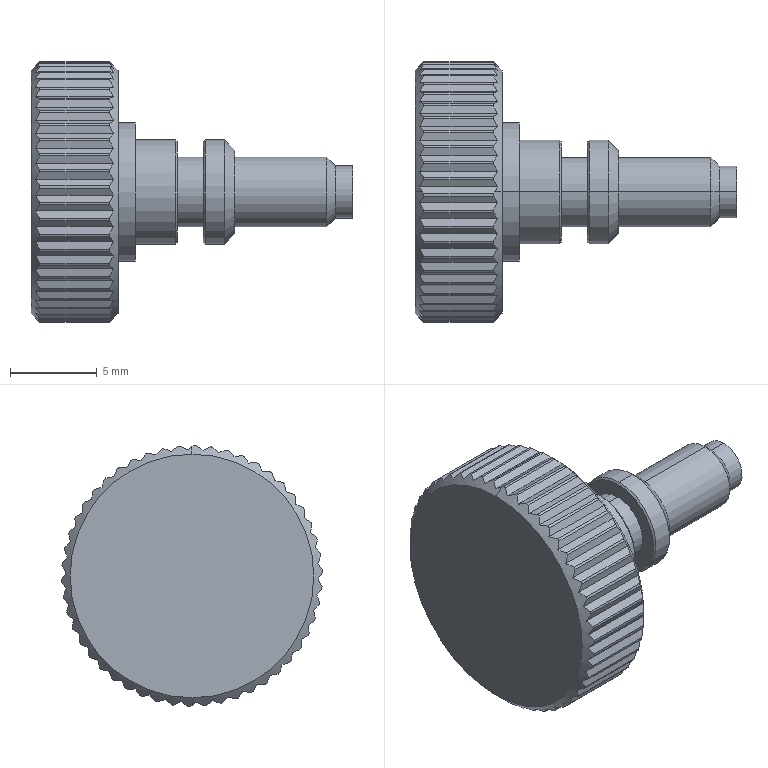Part | SolidWorks | features BaseBody 1 | 1 solid | 181 faces | box 18.5 x 14.994 x 14.998 mm | volume 1115 mm3 | plane 107 | cylinder 62 | cone 12 | commonest cylinder face diameters 15 x50 4 x4 6 x4 3 x2 8 x2